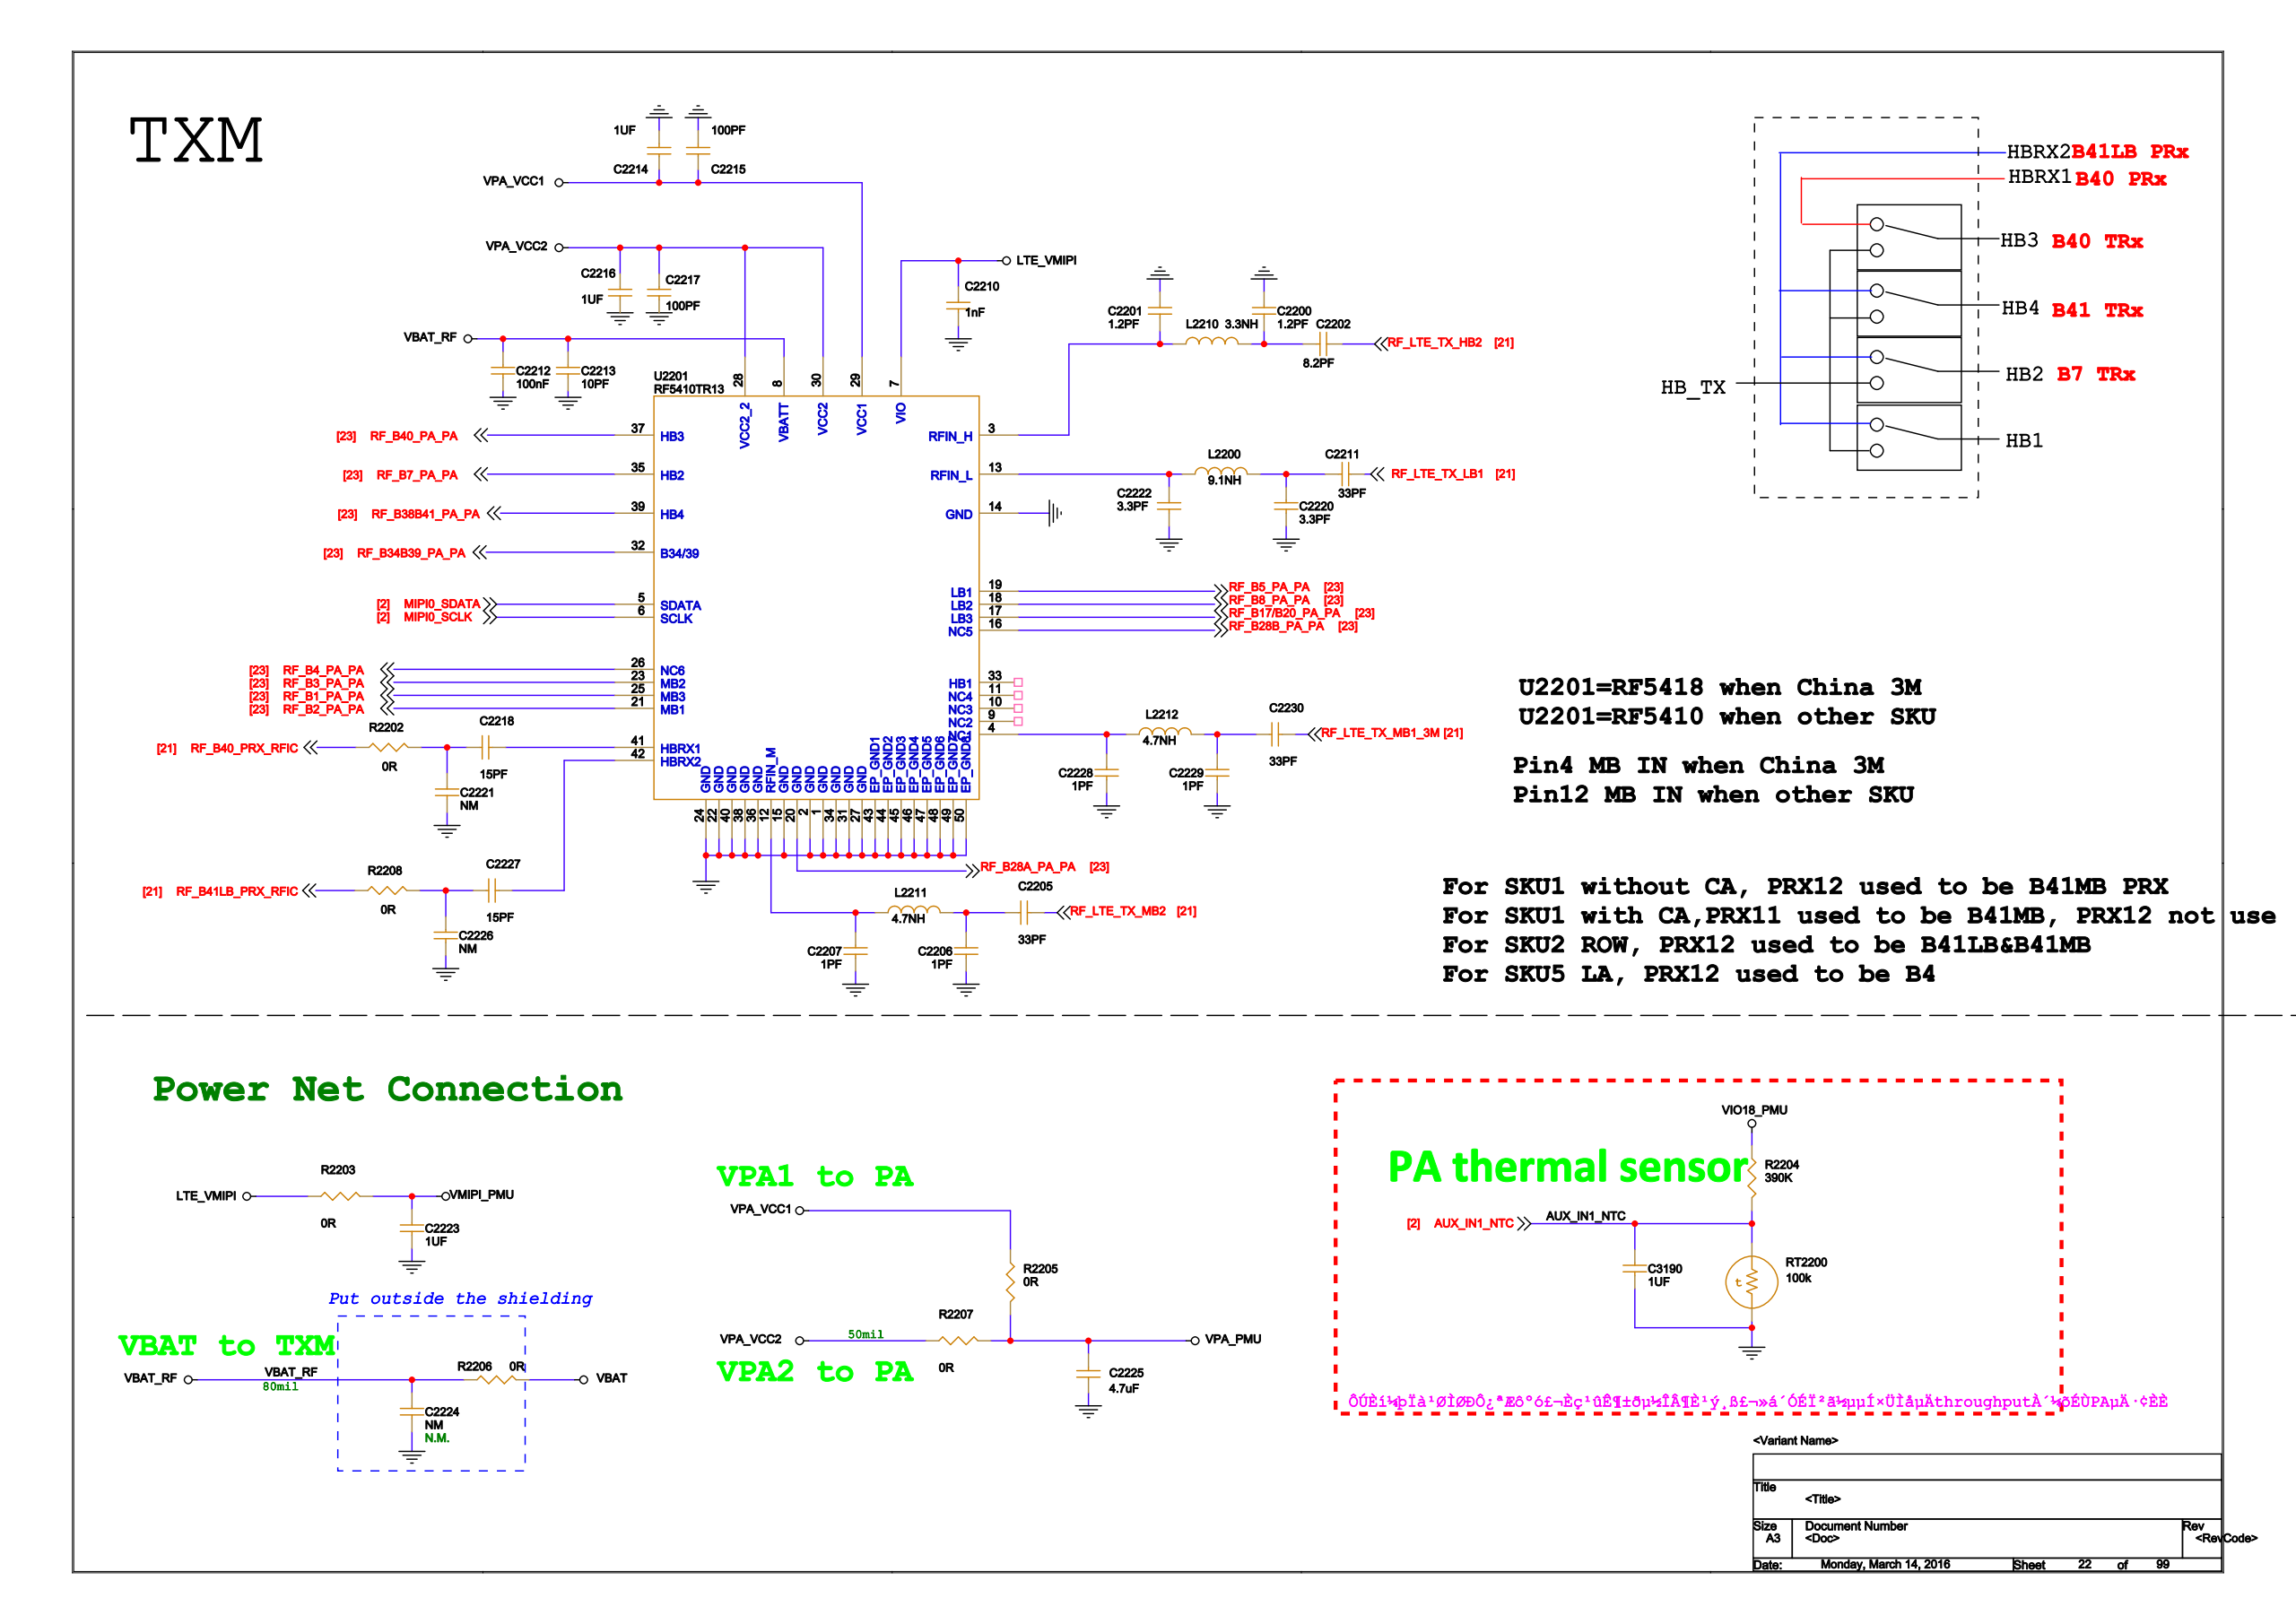Circuit board | Cadence Allegro | 1088 parts | 793 nets | one sheet of the schematic
Parts on this sheet (reference | value | footprint):
C2200 | 1.2PF | C0201
C2201 | 1.2PF | C0201
C2202 | 8.2PF | C0201
C2205 | 33PF | C0201
C2206 | 1PF | C0201
C2207 | 1PF | C0201
C2210 | 1nF | C0201
C2211 | 33PF | C0201
C2212 | 100NF | C0201
C2213 | 10PF | C0201
C2214 | 1UF | C0201
C2215 | 100PF | C0201
C2216 | 1UF | C0201
C2217 | 100PF | C0201
C2218 | 15PF | C0201
C2220 | 3.3PF | C0201
C2221 | NM | 0201_NM
C2222 | 3.3PF | C0201
C2223 | 1UF | C0201
C2224
C2225 | 4.7uF | 0402-BIG
C2226 | NM | 0201_NM
C2227 | 15PF | C0201
C2228 | 1PF | C0201
C2229 | 1PF | C0201
C2230 | 33PF | C0201
C3190 | 1UF | C0201
L2200 | 9.1NH | L0201
L2210 | 3.3NH | L0201
L2211 | 4.7NH | L0201
L2212 | 4.7NH | L0201
R2202 | 0R | R0201
R2203 | 0R | R0201
R2204 | 390K | R0201
R2205 | 0R | R0201
R2206 | 0R | R0603
R2207 | 0R | R0402
R2208 | 0R | R0201
RT2200 | 100k | R0201
U2201 | RF5410TR13 | RF5410
Nets of these parts (net: part-pin ...):
GND: C2200-1 C2201-1 C2206-2 C2207-2 C2210-2 C2212-2 C2213-2 C2214-2 C2215-2 C2216-2 C2217-2 C2220-2 C2221-2 C2222-2 C2223-2 C2224-2 C2225-1 C2226-2 C2228-2 C2229-2 C3190-2 RT2200-2 U2201-1 U2201-2 U2201-14 U2201-15 U2201-22 U2201-24 U2201-27 U2201-31 U2201-34 U2201-36 U2201-38 U2201-40 U2201-43 U2201-44 U2201-45 U2201-46 U2201-47 U2201-48 U2201-49 U2201-50
VBAT: R2206-2
VMIPI_PMU: C2223-1 R2203-2
AUX_IN1_NTC: C3190-1 R2204-2 RT2200-1
MIPI0_SCLK: U2201-6
MIPI0_SDATA: U2201-5
VIO18_PMU: R2204-1
RF_B34B39_PA_PA: U2201-32
RF_B28A_PA_PA: U2201-20
RF_B7_PA_PA: U2201-35
RF_B40_PA_PA: U2201-37
RF_B38B41_PA_PA: U2201-39
N33417819: C2218-2 U2201-41
N33554774: C2227-2 U2201-42
RF_B5_PA_PA: U2201-19
RF_B8_PA_PA: U2201-18
RF_B17/B20_PA_PA: U2201-17
RF_B2_PA_PA: U2201-21
RF_B3_PA_PA: U2201-23
RF_B1_PA_PA: U2201-25
N34534337: C2228-1 L2212-2 U2201-4
RF_B28B_PA_PA: U2201-16
RF_B4_PA_PA: U2201-26
N33422412: C2201-2 L2210-1 U2201-3
N33423439: C2222-1 L2200-1 U2201-13
N33417011: C2207-1 L2211-2 U2201-12
VBAT_RF: C2212-1 C2213-1 C2224-1 R2206-1 U2201-8
VPA_VCC1: C2214-1 C2215-1 R2205-1 U2201-29
VPA_VCC2: C2216-1 C2217-1 R2207-1 U2201-28 U2201-30
LTE_VMIPI: C2210-1 R2203-1 U2201-7
VPA_PMU: C2225-2 R2205-2 R2207-2
N34534339: C2229-1 C2230-1 L2212-1
RF_LTE_TX_MB1_3M: C2230-2
N33417009: C2205-1 C2206-1 L2211-1
RF_LTE_TX_MB2: C2205-2
RF_LTE_TX_LB1: C2211-1
N33423105: C2211-2 C2220-1 L2200-2
N33417817: C2218-1 C2221-1 R2202-2
N33554771: C2226-1 C2227-1 R2208-2
N33451364: C2200-2 C2202-2 L2210-2
RF_LTE_TX_HB2: C2202-1
RF_B40_PRX_RFIC: R2202-1
RF_B41LB_PRX_RFIC: R2208-1